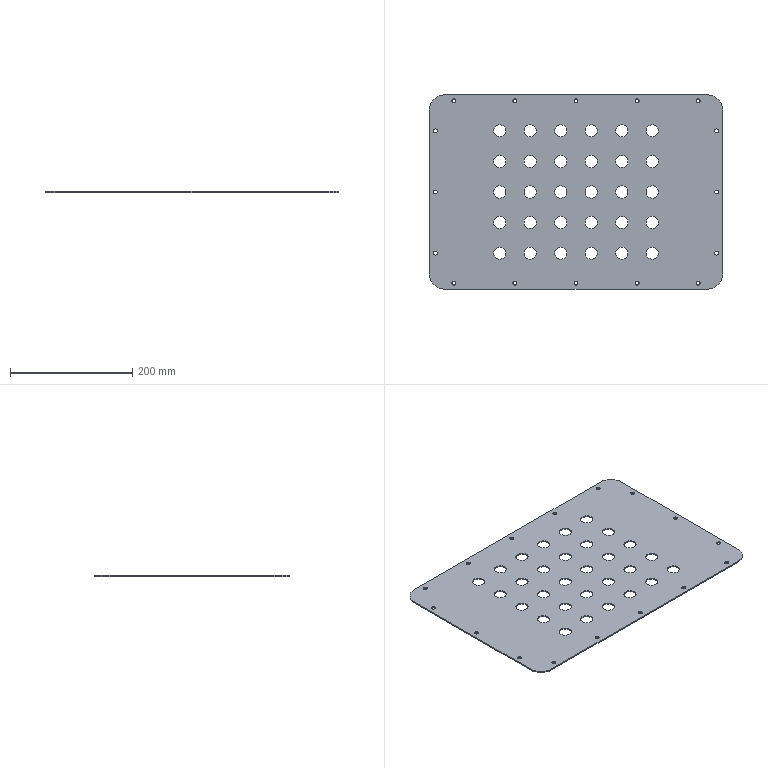Part | SolidWorks | features ICE 2, BaseBody 1 | 1 solid | 102 faces | box 480 x 318 x 2 mm | volume 284296 mm3 | cylinder 96 | plane 6 | commonest cylinder face diameters 20 x60 6.5 x32 50 x4